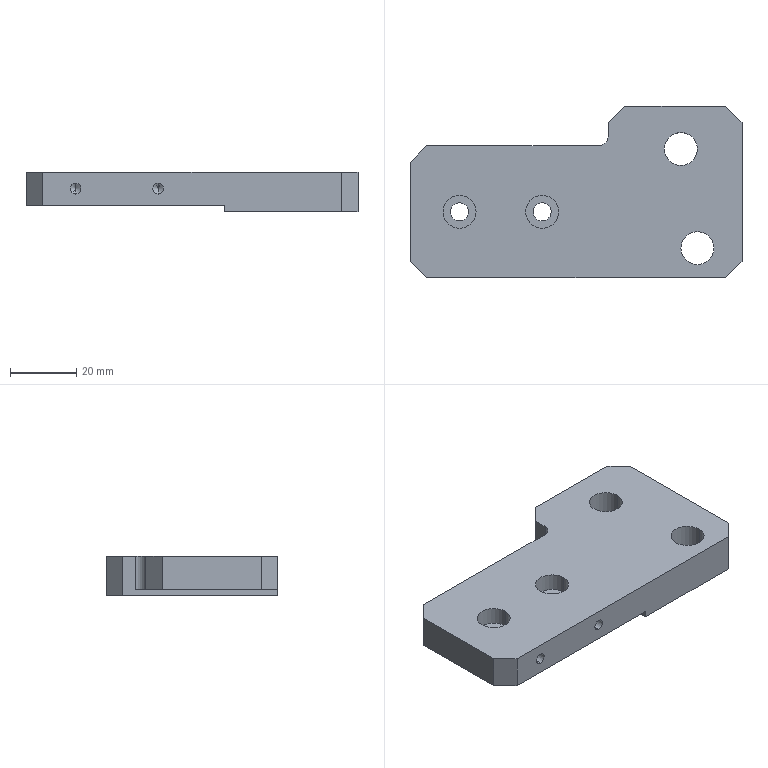Part | STEP file | (PA01.001.LX011) Idler Mounting Plate | 1 solid | 53 faces | box 100.5 x 52 x 12 mm | volume 45032 mm3 | cylinder 25 | plane 16 | cone 12 | commonest cylinder face diameters 3.3 x12 10 x8 5.5 x4 6 x1